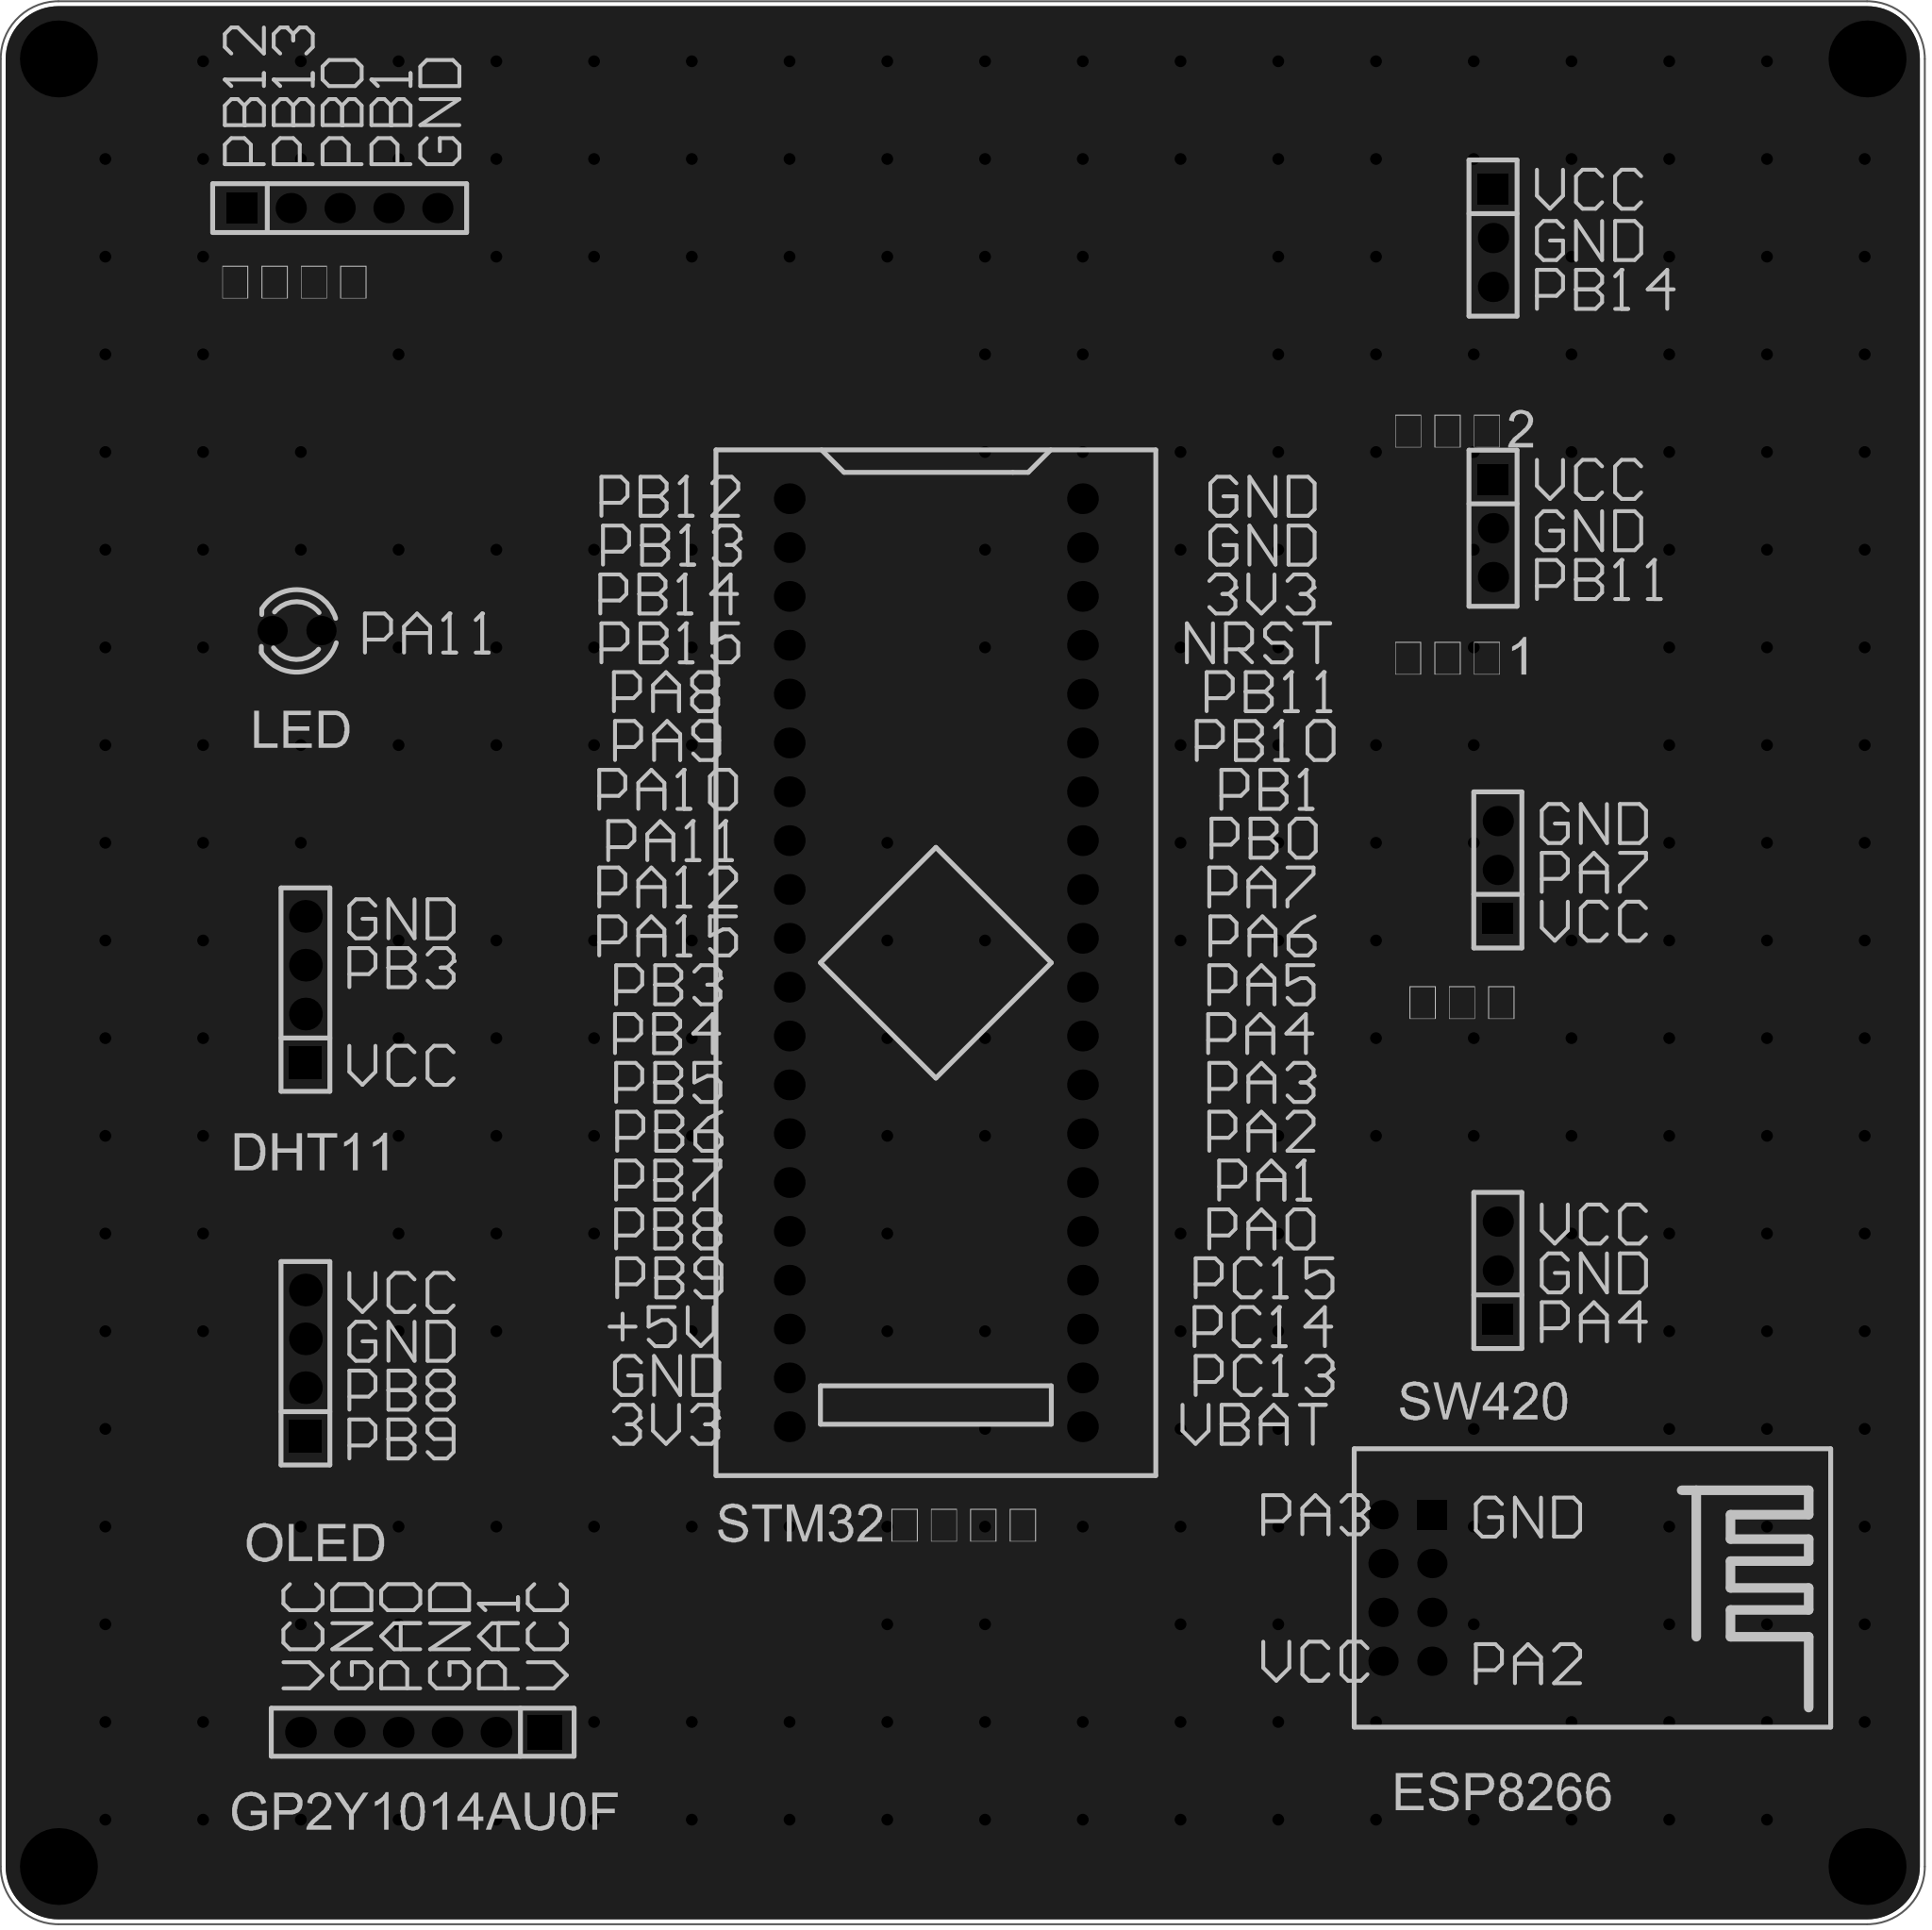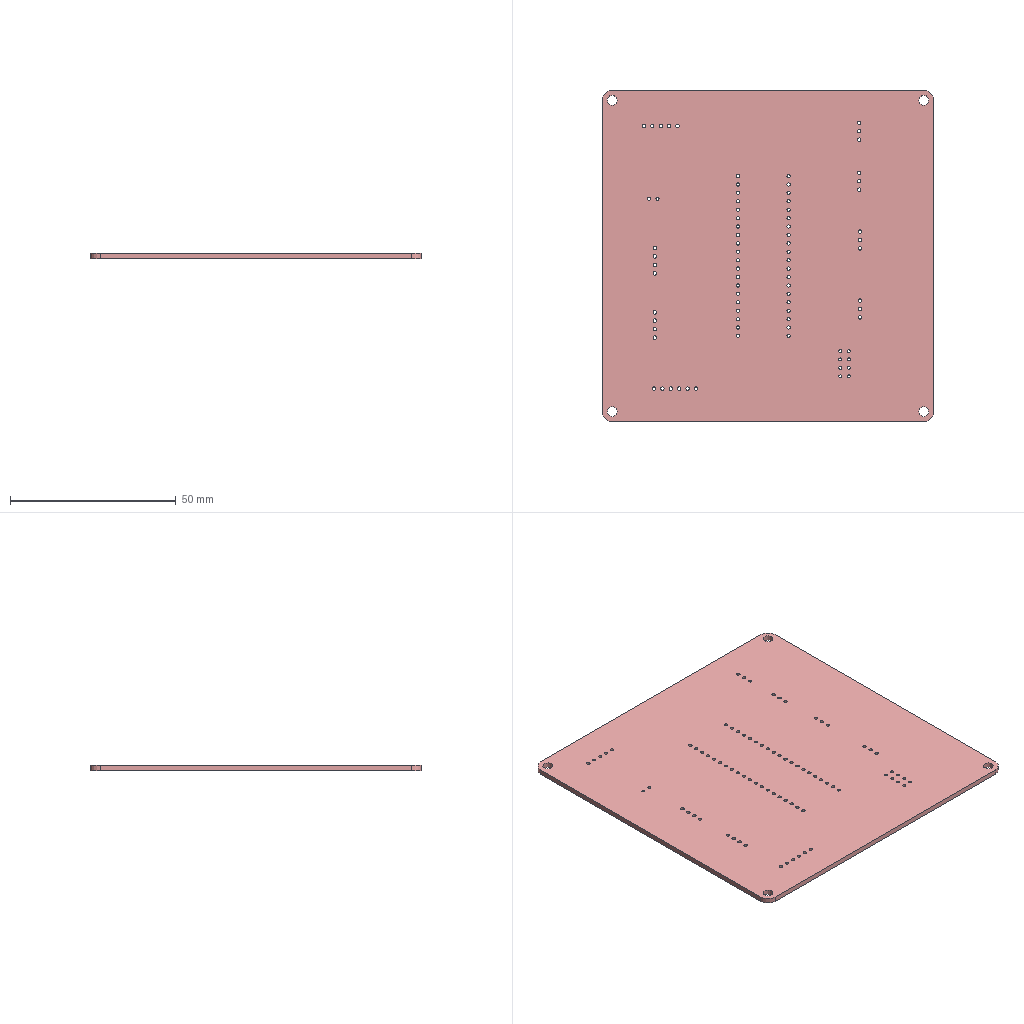Circuit board layout | Altium Designer | box 100 x 100 x 1.6 mm
Layer stack:
# Altium Designer layer stack of  (unit mm; dielectric type: 0 none, 1 core, 2 prepreg, 3 surface material)
index,name,kind,layer,copper_thickness_mm,dielectric_type,dielectric_thickness_mm,dielectric_material,dielectric_constant
0,Top Paste Mask Layer,other,,,,,,
1,Top Silkscreen Layer,other,,,,,,
2,Top Solder Mask Layer,dielectric,,,3,0.01,,3.3
3,Top Layer,copper,Top Layer,0.035,,,,
4,Dielectric1,dielectric,,,3,1.51,FR4,4.5
5,Bottom Layer,copper,Bottom Layer,0.035,,,,
6,Bottom Solder Mask Layer,dielectric,,,3,0.01,,3.3
7,Bottom Silkscreen Layer,other,,,,,,
8,Bottom Paste Mask Layer,other,,,,,,
# drill layer pairs: low layer,high layer
drill_pair,Top Layer,Bottom Layer
Part placement:
Designator,Comment,Layer,Footprint,Center-X(mm),Center-Y(mm),Rotation
U1,STM32F103C8T6-Card,TopLayer,CONN-TH_L53.3-W22.9_STM32F103C8T6-CARD,129.159,128.905,270
H3,,TopLayer,HDR-TH_5P-P2.54-V-F,98.171,168.148,0
H4,,TopLayer,HDR-TH_4P-P2.54-V-F,96.393,127.508,90
H5,,TopLayer,HDR-TH_3P-P2.54-V-F,158.365,112.903,90
H6,,TopLayer,HDR-TH_3P-P2.54-V-F,158.365,133.732,90
H7,,TopLayer,HDR-TH_6P-P2.54-V-F,102.486,88.891,180
H23,,TopLayer,HDR-TH_4P-P2.54-V-F,96.393,108.077,90
LED1,,TopLayer,LED_TH-3mm,95.933,146.177,180
U3,ESP8266-01S,TopLayer,WIFIM-TH_ESP8266-01S,153.67,96.393,270
H1,,TopLayer,HDR-TH_3P-P2.54-V-F,158.115,151.501,270
H2,,TopLayer,HDR-TH_3P-P2.54-V-F,158.115,166.59,270
Pad and via stacks:
# Altium Designer via and pad stacks of  (unit mm). Each distinct definition once, with the count of objects using it.
# via: kind,start_layer,end_layer,hole_mm,diameter_mm,mode(0 simple;1 top-mid-bottom;2 full stack),diameter_per_layer,count,example_net
# pad: kind,layer,hole_mm,hole_type(0 round;1 square;2 slot),plating,top_size,top_shape(1 round;2 rect;3 octagon;9 rounded rect),mid_size,bottom_size,mode,footprint,size_per_layer,count,example
pad,Multi-Layer,3,0,plated,4x4,1,4x4,4x4,0,,,4,1
pad,Multi-Layer,1,0,plated,1.6x1.6,1,1.6x1.6,1.6x1.6,0,CONN-TH_L53.3-W22.9_STM32F103C8T6-CARD,,40,U1.1
pad,Multi-Layer,1.02,0,plated,1.575x1.575,1,1.575x1.575,1.575x1.575,0,HDR-TH_5P-P2.54-V-F,,4,H3.5
pad,Multi-Layer,1.02,0,plated,1.575x1.575,2,1.575x1.575,1.575x1.575,0,HDR-TH_5P-P2.54-V-F,,1,H3.1
pad,Multi-Layer,1.1,0,plated,1.7x1.7,2,1.7x1.7,1.7x1.7,0,HDR-TH_4P-P2.54-V-F,,2,H4.1
pad,Multi-Layer,1.1,0,plated,1.7x1.7,1,1.7x1.7,1.7x1.7,0,HDR-TH_4P-P2.54-V-F,,6,H4.2
pad,Multi-Layer,1.02,0,plated,1.575x1.575,1,1.575x1.575,1.575x1.575,0,HDR-TH_3P-P2.54-V-F,,8,H5.3
pad,Multi-Layer,1.02,0,plated,1.575x1.575,2,1.575x1.575,1.575x1.575,0,HDR-TH_3P-P2.54-V-F,,4,H5.1
pad,Multi-Layer,1.02,0,plated,1.6x1.6,1,1.6x1.6,1.6x1.6,0,HDR-TH_6P-P2.54-V-F,,5,H7.6
pad,Multi-Layer,1.02,0,plated,1.8x1.8,2,1.8x1.8,1.8x1.8,0,HDR-TH_6P-P2.54-V-F,,1,H7.1
pad,Multi-Layer,0.9144,0,plated,1.524x1.524,1,1.524x1.524,1.524x1.524,0,LED_TH-3mm,,2,LED1.1
pad,Multi-Layer,0.9144,0,plated,1.524x1.524,1,1.524x1.524,1.524x1.524,0,WIFIM-TH_ESP8266-01S,,7,U3.8
pad,Multi-Layer,0.9144,0,plated,1.524x1.524,2,1.524x1.524,1.524x1.524,0,WIFIM-TH_ESP8266-01S,,1,U3.1
via,Top Layer,Bottom Layer,0.3048,0.61,0,,264,GND
Copper pours:
name,layer,net,type(0 solid;1 hatched;2 none)
Bottom Layer-GND,Bottom Layer,GND,0
Top Layer-GND,Top Layer,GND,0
Design rules, without the lines most boards share:
# Altium Designer design rules of  (exported by Altium Designer, unit mm)
# columns: name | kind | enabled | priority | scope1 | scope2 | descriptor | typed fields (field=value)
copperThickness1oz_2 | 2 | enabled | 2 | All | All | Width Constraint (Min=5mil) (Max=100mil) (Preferred=30mil) (All) |
viaSize | 11 | enabled | 1 | All | All | Routing Via (MinHoleWidth=11.811mil) (MaxHoleWidth=248.032mil) (PreferredHoleWidth=12.008mil) (MinWidth=19.685mil) (MaxWidth=393.701mil) (PreferedWidth=24.016mil) (All) | via_min_hole=0.3 via_max_hole=6.3 via_preferred_diameter=0.61 via_preferred_hole=0.305
solderMaskExpansion | 13 | enabled | 2 | All | All | Solder Mask Expansion (Expansion =2.008mil) (All) | expansion=0.051